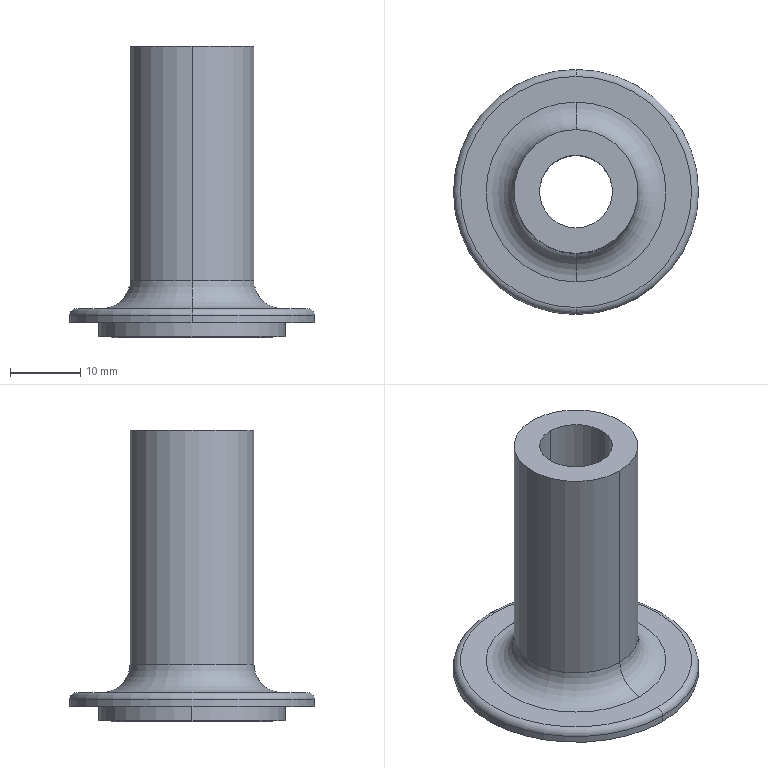Part | SolidWorks | features BaseBody 1 | 1 solid | 51 faces | box 35 x 35 x 41.7 mm | volume 8862 mm3 | torus 22 | cone 14 | cylinder 8 | plane 7 | commonest cylinder face diameters 10.4 x2 17.7 x2 26.6 x2 35 x2
STEP:
#1=CARTESIAN_POINT('',(1903.,34.85,823.));
#2=VERTEX_POINT('',#1);
#3=CARTESIAN_POINT('',(1903.,9.15,823.));
#4=VERTEX_POINT('',#3);
#5=CARTESIAN_POINT('',(1903.,22.,823.));
#6=DIRECTION('',(0.,0.,1.));
#7=DIRECTION('',(0.,1.,0.));
#8=AXIS2_PLACEMENT_3D('',#5,#6,#7);
#9=CIRCLE('',#8,12.85);
#10=EDGE_CURVE('',#2,#4,#9,.T.);
#11=ORIENTED_EDGE('',*,*,#10,.T.);
#12=CARTESIAN_POINT('',(1903.,13.15,827.));
#13=VERTEX_POINT('',#12);
#14=CARTESIAN_POINT('',(1903.,9.15,827.));
#15=DIRECTION('',(1.,0.,0.));
#16=DIRECTION('',(0.,1.,0.));
#17=AXIS2_PLACEMENT_3D('',#14,#15,#16);
#18=CIRCLE('',#17,4.);
#19=EDGE_CURVE('',#4,#13,#18,.T.);
#20=ORIENTED_EDGE('',*,*,#19,.T.);
#21=CARTESIAN_POINT('',(1903.,30.85,827.));
#22=VERTEX_POINT('',#21);
#23=CARTESIAN_POINT('',(1903.,22.,827.));
#24=DIRECTION('',(0.,0.,1.));
#25=DIRECTION('',(0.,1.,0.));
#26=AXIS2_PLACEMENT_3D('',#23,#24,#25);
#27=CIRCLE('',#26,8.85);
#28=EDGE_CURVE('',#22,#13,#27,.T.);
#29=ORIENTED_EDGE('',*,*,#28,.F.);
#30=CARTESIAN_POINT('',(1903.,34.85,827.));
#31=DIRECTION('',(1.,0.,0.));
#32=DIRECTION('',(0.,-1.,0.));
#33=AXIS2_PLACEMENT_3D('',#30,#31,#32);
#34=CIRCLE('',#33,4.);
#35=EDGE_CURVE('',#22,#2,#34,.T.);
#36=ORIENTED_EDGE('',*,*,#35,.T.);
#37=EDGE_LOOP('',(#11,#20,#29,#36));
#38=FACE_OUTER_BOUND('',#37,.T.);
#39=CARTESIAN_POINT('',(1903.,22.,827.));
#40=DIRECTION('',(0.,0.,1.));
#41=DIRECTION('',(0.,1.,0.));
#42=AXIS2_PLACEMENT_3D('',#39,#40,#41);
#43=TOROIDAL_SURFACE('',#42,12.85,4.);
#44=ADVANCED_FACE('',(#38),#43,.F.);
#45=CARTESIAN_POINT('',(1903.,22.,827.));
#46=DIRECTION('',(0.,0.,-1.));
#47=DIRECTION('',(0.,1.,0.));
#48=AXIS2_PLACEMENT_3D('',#45,#46,#47);
#49=CIRCLE('',#48,8.85);
#50=EDGE_CURVE('',#22,#13,#49,.T.);
#51=ORIENTED_EDGE('',*,*,#50,.T.);
#52=ORIENTED_EDGE('',*,*,#19,.F.);
#53=CARTESIAN_POINT('',(1903.,22.,823.));
#54=DIRECTION('',(0.,0.,-1.));
#55=DIRECTION('',(0.,1.,0.));
#56=AXIS2_PLACEMENT_3D('',#53,#54,#55);
#57=CIRCLE('',#56,12.85);
#58=EDGE_CURVE('',#2,#4,#57,.T.);
#59=ORIENTED_EDGE('',*,*,#58,.F.);
#60=ORIENTED_EDGE('',*,*,#35,.F.);
#61=EDGE_LOOP('',(#51,#52,#59,#60));
#62=FACE_OUTER_BOUND('',#61,.T.);
#63=CARTESIAN_POINT('',(1903.,22.,827.));
#64=DIRECTION('',(0.,0.,1.));
#65=DIRECTION('',(0.,1.,0.));
#66=AXIS2_PLACEMENT_3D('',#63,#64,#65);
#67=TOROIDAL_SURFACE('',#66,12.85,4.);
#68=ADVANCED_FACE('',(#62),#67,.F.);
#69=CARTESIAN_POINT('',(1903.,38.5,823.));
#70=VERTEX_POINT('',#69);
#71=CARTESIAN_POINT('',(1903.,5.5,823.));
#72=VERTEX_POINT('',#71);
#73=CARTESIAN_POINT('',(1903.,22.,823.));
#74=DIRECTION('',(0.,0.,-1.));
#75=DIRECTION('',(0.,1.,0.));
#76=AXIS2_PLACEMENT_3D('',#73,#74,#75);
#77=CIRCLE('',#76,16.5);
#78=EDGE_CURVE('',#70,#72,#77,.T.);
#79=ORIENTED_EDGE('',*,*,#78,.F.);
#80=CARTESIAN_POINT('',(1903.,22.,823.));
#81=DIRECTION('',(0.,0.,1.));
#82=DIRECTION('',(0.,1.,0.));
#83=AXIS2_PLACEMENT_3D('',#80,#81,#82);
#84=CIRCLE('',#83,16.5);
#85=EDGE_CURVE('',#70,#72,#84,.T.);
#86=ORIENTED_EDGE('',*,*,#85,.T.);
#87=EDGE_LOOP('',(#79,#86));
#88=FACE_OUTER_BOUND('',#87,.T.);
#89=ORIENTED_EDGE('',*,*,#10,.F.);
#90=ORIENTED_EDGE('',*,*,#58,.T.);
#91=EDGE_LOOP('',(#89,#90));
#92=FACE_BOUND('',#91,.T.);
#93=CARTESIAN_POINT('',(1903.,22.,823.));
#94=DIRECTION('',(0.,0.,1.));
#95=DIRECTION('',(0.,1.,0.));
#96=AXIS2_PLACEMENT_3D('',#93,#94,#95);
#97=PLANE('',#96);
#98=ADVANCED_FACE('',(#88,#92),#97,.T.);
#99=CARTESIAN_POINT('',(1903.,39.5,822.));
#100=VERTEX_POINT('',#99);
#101=CARTESIAN_POINT('',(1903.,4.5,822.));
#102=VERTEX_POINT('',#101);
#103=CARTESIAN_POINT('',(1903.,22.,822.));
#104=DIRECTION('',(0.,0.,1.));
#105=DIRECTION('',(0.,1.,0.));
#106=AXIS2_PLACEMENT_3D('',#103,#104,#105);
#107=CIRCLE('',#106,17.5);
#108=EDGE_CURVE('',#100,#102,#107,.T.);
#109=ORIENTED_EDGE('',*,*,#108,.T.);
#110=CARTESIAN_POINT('',(1903.,5.5,822.));
#111=DIRECTION('',(-1.,0.,0.));
#112=DIRECTION('',(0.,0.,1.));
#113=AXIS2_PLACEMENT_3D('',#110,#111,#112);
#114=CIRCLE('',#113,1.);
#115=EDGE_CURVE('',#102,#72,#114,.T.);
#116=ORIENTED_EDGE('',*,*,#115,.T.);
#117=ORIENTED_EDGE('',*,*,#85,.F.);
#118=CARTESIAN_POINT('',(1903.,38.5,822.));
#119=DIRECTION('',(-1.,0.,0.));
#120=DIRECTION('',(0.,0.,1.));
#121=AXIS2_PLACEMENT_3D('',#118,#119,#120);
#122=CIRCLE('',#121,1.);
#123=EDGE_CURVE('',#70,#100,#122,.T.);
#124=ORIENTED_EDGE('',*,*,#123,.T.);
#125=EDGE_LOOP('',(#109,#116,#117,#124));
#126=FACE_OUTER_BOUND('',#125,.T.);
#127=CARTESIAN_POINT('',(1903.,22.,822.));
#128=DIRECTION('',(0.,0.,1.));
#129=DIRECTION('',(0.,1.,0.));
#130=AXIS2_PLACEMENT_3D('',#127,#128,#129);
#131=TOROIDAL_SURFACE('',#130,16.5,1.);
#132=ADVANCED_FACE('',(#126),#131,.T.);
#133=ORIENTED_EDGE('',*,*,#78,.T.);
#134=ORIENTED_EDGE('',*,*,#115,.F.);
#135=CARTESIAN_POINT('',(1903.,22.,822.));
#136=DIRECTION('',(0.,0.,-1.));
#137=DIRECTION('',(0.,1.,0.));
#138=AXIS2_PLACEMENT_3D('',#135,#136,#137);
#139=CIRCLE('',#138,17.5);
#140=EDGE_CURVE('',#100,#102,#139,.T.);
#141=ORIENTED_EDGE('',*,*,#140,.F.);
#142=ORIENTED_EDGE('',*,*,#123,.F.);
#143=EDGE_LOOP('',(#133,#134,#141,#142));
#144=FACE_OUTER_BOUND('',#143,.T.);
#145=CARTESIAN_POINT('',(1903.,22.,822.));
#146=DIRECTION('',(0.,0.,1.));
#147=DIRECTION('',(0.,1.,0.));
#148=AXIS2_PLACEMENT_3D('',#145,#146,#147);
#149=TOROIDAL_SURFACE('',#148,16.5,1.);
#150=ADVANCED_FACE('',(#144),#149,.T.);
#151=CARTESIAN_POINT('',(1903.,39.5,821.));
#152=VERTEX_POINT('',#151);
#153=CARTESIAN_POINT('',(1903.,39.5,822.));
#154=DIRECTION('',(0.,0.,1.));
#155=VECTOR('',#154,1000.);
#156=LINE('',#153,#155);
#157=EDGE_CURVE('',#152,#100,#156,.T.);
#158=ORIENTED_EDGE('',*,*,#157,.T.);
#159=ORIENTED_EDGE('',*,*,#140,.T.);
#160=CARTESIAN_POINT('',(1903.,4.5,821.));
#161=VERTEX_POINT('',#160);
#162=CARTESIAN_POINT('',(1903.,4.5,822.));
#163=DIRECTION('',(0.,0.,-1.));
#164=VECTOR('',#163,1000.);
#165=LINE('',#162,#164);
#166=EDGE_CURVE('',#102,#161,#165,.T.);
#167=ORIENTED_EDGE('',*,*,#166,.T.);
#168=CARTESIAN_POINT('',(1903.,22.,821.));
#169=DIRECTION('',(0.,0.,-1.));
#170=DIRECTION('',(0.,1.,0.));
#171=AXIS2_PLACEMENT_3D('',#168,#169,#170);
#172=CIRCLE('',#171,17.5);
#173=EDGE_CURVE('',#152,#161,#172,.T.);
#174=ORIENTED_EDGE('',*,*,#173,.F.);
#175=EDGE_LOOP('',(#158,#159,#167,#174));
#176=FACE_OUTER_BOUND('',#175,.T.);
#177=CARTESIAN_POINT('',(1903.,22.,816.925));
#178=DIRECTION('',(0.,0.,1.));
#179=DIRECTION('',(0.,1.,0.));
#180=AXIS2_PLACEMENT_3D('',#177,#178,#179);
#181=CYLINDRICAL_SURFACE('',#180,17.5);
#182=ADVANCED_FACE('',(#176),#181,.T.);
#183=ORIENTED_EDGE('',*,*,#173,.T.);
#184=CARTESIAN_POINT('',(1903.,22.,821.));
#185=DIRECTION('',(0.,0.,-1.));
#186=DIRECTION('',(0.,-1.,0.));
#187=AXIS2_PLACEMENT_3D('',#184,#185,#186);
#188=CIRCLE('',#187,17.5);
#189=EDGE_CURVE('',#161,#152,#188,.T.);
#190=ORIENTED_EDGE('',*,*,#189,.T.);
#191=EDGE_LOOP('',(#183,#190));
#192=FACE_OUTER_BOUND('',#191,.T.);
#193=CARTESIAN_POINT('',(1916.3,22.,821.));
#194=VERTEX_POINT('',#193);
#195=CARTESIAN_POINT('',(1889.7,22.,821.));
#196=VERTEX_POINT('',#195);
#197=CARTESIAN_POINT('',(1903.,22.,821.));
#198=DIRECTION('',(0.,0.,1.));
#199=DIRECTION('',(1.,0.,0.));
#200=AXIS2_PLACEMENT_3D('',#197,#198,#199);
#201=CIRCLE('',#200,13.3);
#202=EDGE_CURVE('',#194,#196,#201,.T.);
#203=ORIENTED_EDGE('',*,*,#202,.T.);
#204=CARTESIAN_POINT('',(1903.,22.,821.));
#205=DIRECTION('',(0.,0.,-1.));
#206=DIRECTION('',(1.,0.,0.));
#207=AXIS2_PLACEMENT_3D('',#204,#205,#206);
#208=CIRCLE('',#207,13.3);
#209=EDGE_CURVE('',#194,#196,#208,.T.);
#210=ORIENTED_EDGE('',*,*,#209,.F.);
#211=EDGE_LOOP('',(#203,#210));
#212=FACE_BOUND('',#211,.T.);
#213=CARTESIAN_POINT('',(1903.,22.,821.));
#214=DIRECTION('',(0.,0.,-1.));
#215=DIRECTION('',(-1.,0.,0.));
#216=AXIS2_PLACEMENT_3D('',#213,#214,#215);
#217=PLANE('',#216);
#218=ADVANCED_FACE('',(#192,#212),#217,.T.);
#219=CARTESIAN_POINT('',(1916.3,22.,819.));
#220=VERTEX_POINT('',#219);
#221=CARTESIAN_POINT('',(1916.3,22.,819.));
#222=DIRECTION('',(0.,0.,-1.));
#223=VECTOR('',#222,1000.);
#224=LINE('',#221,#223);
#225=EDGE_CURVE('',#194,#220,#224,.T.);
#226=ORIENTED_EDGE('',*,*,#225,.F.);
#227=ORIENTED_EDGE('',*,*,#209,.T.);
#228=CARTESIAN_POINT('',(1889.7,22.,819.));
#229=VERTEX_POINT('',#228);
#230=CARTESIAN_POINT('',(1889.7,22.,819.));
#231=DIRECTION('',(0.,0.,1.));
#232=VECTOR('',#231,1000.);
#233=LINE('',#230,#232);
#234=EDGE_CURVE('',#229,#196,#233,.T.);
#235=ORIENTED_EDGE('',*,*,#234,.F.);
#236=CARTESIAN_POINT('',(1903.,22.,819.));
#237=DIRECTION('',(0.,0.,-1.));
#238=DIRECTION('',(1.,0.,0.));
#239=AXIS2_PLACEMENT_3D('',#236,#237,#238);
#240=CIRCLE('',#239,13.3);
#241=EDGE_CURVE('',#220,#229,#240,.T.);
#242=ORIENTED_EDGE('',*,*,#241,.F.);
#243=EDGE_LOOP('',(#226,#227,#235,#242));
#244=FACE_OUTER_BOUND('',#243,.T.);
#245=CARTESIAN_POINT('',(1903.,22.,821.1));
#246=DIRECTION('',(0.,0.,-1.));
#247=DIRECTION('',(-1.,0.,0.));
#248=AXIS2_PLACEMENT_3D('',#245,#246,#247);
#249=CYLINDRICAL_SURFACE('',#248,13.3);
#250=ADVANCED_FACE('',(#244),#249,.T.);
#251=CARTESIAN_POINT('',(1903.,22.,819.));
#252=DIRECTION('',(0.,0.,-1.));
#253=DIRECTION('',(-1.,0.,0.));
#254=AXIS2_PLACEMENT_3D('',#251,#252,#253);
#255=CIRCLE('',#254,13.3);
#256=EDGE_CURVE('',#229,#220,#255,.T.);
#257=ORIENTED_EDGE('',*,*,#256,.T.);
#258=ORIENTED_EDGE('',*,*,#241,.T.);
#259=EDGE_LOOP('',(#257,#258));
#260=FACE_OUTER_BOUND('',#259,.T.);
#261=CARTESIAN_POINT('',(1891.327,22.,819.));
#262=VERTEX_POINT('',#261);
#263=CARTESIAN_POINT('',(1914.673,22.,819.));
#264=VERTEX_POINT('',#263);
#265=CARTESIAN_POINT('',(1903.,22.,819.));
#266=DIRECTION('',(0.,0.,1.));
#267=DIRECTION('',(-1.,0.,0.));
#268=AXIS2_PLACEMENT_3D('',#265,#266,#267);
#269=CIRCLE('',#268,11.673);
#270=EDGE_CURVE('',#262,#264,#269,.T.);
#271=ORIENTED_EDGE('',*,*,#270,.T.);
#272=CARTESIAN_POINT('',(1903.,22.,819.));
#273=DIRECTION('',(0.,0.,1.));
#274=DIRECTION('',(1.,0.,0.));
#275=AXIS2_PLACEMENT_3D('',#272,#273,#274);
#276=CIRCLE('',#275,11.673);
#277=EDGE_CURVE('',#264,#262,#276,.T.);
#278=ORIENTED_EDGE('',*,*,#277,.T.);
#279=EDGE_LOOP('',(#271,#278));
#280=FACE_BOUND('',#279,.T.);
#281=CARTESIAN_POINT('',(1903.,22.,819.));
#282=DIRECTION('',(0.,0.,1.));
#283=DIRECTION('',(0.,1.,0.));
#284=AXIS2_PLACEMENT_3D('',#281,#282,#283);
#285=PLANE('',#284);
#286=ADVANCED_FACE('',(#260,#280),#285,.F.);
#287=CARTESIAN_POINT('',(1891.673,22.,819.));
#288=VERTEX_POINT('',#287);
#289=CARTESIAN_POINT('',(1914.327,22.,819.));
#290=VERTEX_POINT('',#289);
#291=CARTESIAN_POINT('',(1903.,22.,819.));
#292=DIRECTION('',(0.,0.,1.));
#293=DIRECTION('',(-1.,0.,0.));
#294=AXIS2_PLACEMENT_3D('',#291,#292,#293);
#295=CIRCLE('',#294,11.327);
#296=EDGE_CURVE('',#288,#290,#295,.T.);
#297=ORIENTED_EDGE('',*,*,#296,.F.);
#298=CARTESIAN_POINT('',(1903.,22.,819.));
#299=DIRECTION('',(0.,0.,1.));
#300=DIRECTION('',(1.,0.,0.));
#301=AXIS2_PLACEMENT_3D('',#298,#299,#300);
#302=CIRCLE('',#301,11.327);
#303=EDGE_CURVE('',#290,#288,#302,.T.);
#304=ORIENTED_EDGE('',*,*,#303,.F.);
#305=EDGE_LOOP('',(#297,#304));
#306=FACE_OUTER_BOUND('',#305,.T.);
#307=CARTESIAN_POINT('',(1893.327,22.,819.));
#308=VERTEX_POINT('',#307);
#309=CARTESIAN_POINT('',(1912.673,22.,819.));
#310=VERTEX_POINT('',#309);
#311=CARTESIAN_POINT('',(1903.,22.,819.));
#312=DIRECTION('',(0.,0.,1.));
#313=DIRECTION('',(-1.,0.,0.));
#314=AXIS2_PLACEMENT_3D('',#311,#312,#313);
#315=CIRCLE('',#314,9.673);
#316=EDGE_CURVE('',#308,#310,#315,.T.);
#317=ORIENTED_EDGE('',*,*,#316,.T.);
#318=CARTESIAN_POINT('',(1903.,22.,819.));
#319=DIRECTION('',(0.,0.,1.));
#320=DIRECTION('',(1.,0.,0.));
#321=AXIS2_PLACEMENT_3D('',#318,#319,#320);
#322=CIRCLE('',#321,9.673);
#323=EDGE_CURVE('',#310,#308,#322,.T.);
#324=ORIENTED_EDGE('',*,*,#323,.T.);
#325=EDGE_LOOP('',(#317,#324));
#326=FACE_BOUND('',#325,.T.);
#327=CARTESIAN_POINT('',(1903.,22.,819.));
#328=DIRECTION('',(0.,0.,1.));
#329=DIRECTION('',(0.,1.,0.));
#330=AXIS2_PLACEMENT_3D('',#327,#328,#329);
#331=PLANE('',#330);
#332=ADVANCED_FACE('',(#306,#326),#331,.F.);
#333=CARTESIAN_POINT('',(1893.673,22.,819.));
#334=VERTEX_POINT('',#333);
#335=CARTESIAN_POINT('',(1912.327,22.,819.));
#336=VERTEX_POINT('',#335);
#337=CARTESIAN_POINT('',(1903.,22.,819.));
#338=DIRECTION('',(0.,0.,1.));
#339=DIRECTION('',(-1.,0.,0.));
#340=AXIS2_PLACEMENT_3D('',#337,#338,#339);
#341=CIRCLE('',#340,9.327);
#342=EDGE_CURVE('',#334,#336,#341,.T.);
#343=ORIENTED_EDGE('',*,*,#342,.F.);
#344=CARTESIAN_POINT('',(1903.,22.,819.));
#345=DIRECTION('',(0.,0.,1.));
#346=DIRECTION('',(1.,0.,0.));
#347=AXIS2_PLACEMENT_3D('',#344,#345,#346);
#348=CIRCLE('',#347,9.327);
#349=EDGE_CURVE('',#336,#334,#348,.T.);
#350=ORIENTED_EDGE('',*,*,#349,.F.);
#351=EDGE_LOOP('',(#343,#350));
#352=FACE_OUTER_BOUND('',#351,.T.);
#353=CARTESIAN_POINT('',(1895.327,22.,819.));
#354=VERTEX_POINT('',#353);
#355=CARTESIAN_POINT('',(1910.673,22.,819.));
#356=VERTEX_POINT('',#355);
#357=CARTESIAN_POINT('',(1903.,22.,819.));
#358=DIRECTION('',(0.,0.,1.));
#359=DIRECTION('',(-1.,0.,0.));
#360=AXIS2_PLACEMENT_3D('',#357,#358,#359);
#361=CIRCLE('',#360,7.673);
#362=EDGE_CURVE('',#354,#356,#361,.T.);
#363=ORIENTED_EDGE('',*,*,#362,.T.);
#364=CARTESIAN_POINT('',(1903.,22.,819.));
#365=DIRECTION('',(0.,0.,1.));
#366=DIRECTION('',(1.,0.,0.));
#367=AXIS2_PLACEMENT_3D('',#364,#365,#366);
#368=CIRCLE('',#367,7.673);
#369=EDGE_CURVE('',#356,#354,#368,.T.);
#370=ORIENTED_EDGE('',*,*,#369,.T.);
#371=EDGE_LOOP('',(#363,#370));
#372=FACE_BOUND('',#371,.T.);
#373=CARTESIAN_POINT('',(1903.,22.,819.));
#374=DIRECTION('',(0.,0.,1.));
#375=DIRECTION('',(0.,1.,0.));
#376=AXIS2_PLACEMENT_3D('',#373,#374,#375);
#377=PLANE('',#376);
#378=ADVANCED_FACE('',(#352,#372),#377,.F.);
#379=CARTESIAN_POINT('',(1895.673,22.,819.));
#380=VERTEX_POINT('',#379);
#381=CARTESIAN_POINT('',(1910.327,22.,819.));
#382=VERTEX_POINT('',#381);
#383=CARTESIAN_POINT('',(1903.,22.,819.));
#384=DIRECTION('',(0.,0.,1.));
#385=DIRECTION('',(-1.,0.,0.));
#386=AXIS2_PLACEMENT_3D('',#383,#384,#385);
#387=CIRCLE('',#386,7.327);
#388=EDGE_CURVE('',#380,#382,#387,.T.);
#389=ORIENTED_EDGE('',*,*,#388,.F.);
#390=CARTESIAN_POINT('',(1903.,22.,819.));
#391=DIRECTION('',(0.,0.,1.));
#392=DIRECTION('',(1.,0.,0.));
#393=AXIS2_PLACEMENT_3D('',#390,#391,#392);
#394=CIRCLE('',#393,7.327);
#395=EDGE_CURVE('',#382,#380,#394,.T.);
#396=ORIENTED_EDGE('',*,*,#395,.F.);
#397=EDGE_LOOP('',(#389,#396));
#398=FACE_OUTER_BOUND('',#397,.T.);
#399=CARTESIAN_POINT('',(1903.,28.,819.));
#400=VERTEX_POINT('',#399);
#401=CARTESIAN_POINT('',(1903.,16.,819.));
#402=VERTEX_POINT('',#401);
#403=CARTESIAN_POINT('',(1903.,22.,819.));
#404=DIRECTION('',(0.,0.,-1.));
#405=DIRECTION('',(0.,1.,0.));
#406=AXIS2_PLACEMENT_3D('',#403,#404,#405);
#407=CIRCLE('',#406,6.);
#408=EDGE_CURVE('',#400,#402,#407,.T.);
#409=ORIENTED_EDGE('',*,*,#408,.F.);
#410=CARTESIAN_POINT('',(1903.,22.,819.));
#411=DIRECTION('',(0.,0.,1.));
#412=DIRECTION('',(0.,1.,0.));
#413=AXIS2_PLACEMENT_3D('',#410,#411,#412);
#414=CIRCLE('',#413,6.);
#415=EDGE_CURVE('',#400,#402,#414,.T.);
#416=ORIENTED_EDGE('',*,*,#415,.T.);
#417=EDGE_LOOP('',(#409,#416));
#418=FACE_BOUND('',#417,.T.);
#419=CARTESIAN_POINT('',(1903.,22.,819.));
#420=DIRECTION('',(0.,0.,1.));
#421=DIRECTION('',(0.,1.,0.));
#422=AXIS2_PLACEMENT_3D('',#419,#420,#421);
#423=PLANE('',#422);
#424=ADVANCED_FACE('',(#398,#418),#423,.F.);
#425=CARTESIAN_POINT('',(1903.,27.2,824.));
#426=VERTEX_POINT('',#425);
#427=CARTESIAN_POINT('',(1903.,16.8,824.));
#428=VERTEX_POINT('',#427);
#429=CARTESIAN_POINT('',(1903.,22.,824.));
#430=DIRECTION('',(0.,0.,1.));
#431=DIRECTION('',(0.,1.,0.));
#432=AXIS2_PLACEMENT_3D('',#429,#430,#431);
#433=CIRCLE('',#432,5.2);
#434=EDGE_CURVE('',#426,#428,#433,.T.);
#435=ORIENTED_EDGE('',*,*,#434,.T.);
#436=CARTESIAN_POINT('',(1903.,16.,819.));
#437=DIRECTION('',(0.,-0.158,-0.9874));
#438=VECTOR('',#437,1000.);
#439=LINE('',#436,#438);
#440=EDGE_CURVE('',#428,#402,#439,.T.);
#441=ORIENTED_EDGE('',*,*,#440,.T.);
#442=ORIENTED_EDGE('',*,*,#415,.F.);
#443=CARTESIAN_POINT('',(1903.,28.,819.));
#444=DIRECTION('',(0.,-0.158,0.9874));
#445=VECTOR('',#444,1000.);
#446=LINE('',#443,#445);
#447=EDGE_CURVE('',#400,#426,#446,.T.);
#448=ORIENTED_EDGE('',*,*,#447,.T.);
#449=EDGE_LOOP('',(#435,#441,#442,#448));
#450=FACE_OUTER_BOUND('',#449,.T.);
#451=CARTESIAN_POINT('',(1903.,22.,821.5));
#452=DIRECTION('',(0.,0.,-1.));
#453=DIRECTION('',(0.,-1.,0.));
#454=AXIS2_PLACEMENT_3D('',#451,#452,#453);
#455=CONICAL_SURFACE('',#454,5.6,0.1587);
#456=ADVANCED_FACE('',(#450),#455,.F.);
#457=ORIENTED_EDGE('',*,*,#408,.T.);
#458=ORIENTED_EDGE('',*,*,#440,.F.);
#459=CARTESIAN_POINT('',(1903.,22.,824.));
#460=DIRECTION('',(0.,0.,-1.));
#461=DIRECTION('',(0.,1.,0.));
#462=AXIS2_PLACEMENT_3D('',#459,#460,#461);
#463=CIRCLE('',#462,5.2);
#464=EDGE_CURVE('',#426,#428,#463,.T.);
#465=ORIENTED_EDGE('',*,*,#464,.F.);
#466=ORIENTED_EDGE('',*,*,#447,.F.);
#467=EDGE_LOOP('',(#457,#458,#465,#466));
#468=FACE_OUTER_BOUND('',#467,.T.);
#469=CARTESIAN_POINT('',(1903.,22.,821.5));
#470=DIRECTION('',(0.,0.,-1.));
#471=DIRECTION('',(0.,-1.,0.));
#472=AXIS2_PLACEMENT_3D('',#469,#470,#471);
#473=CONICAL_SURFACE('',#472,5.6,0.1587);
#474=ADVANCED_FACE('',(#468),#473,.F.);
#475=ORIENTED_EDGE('',*,*,#464,.T.);
#476=CARTESIAN_POINT('',(1903.,16.8,860.5));
#477=VERTEX_POINT('',#476);
#478=CARTESIAN_POINT('',(1903.,16.8,824.));
#479=DIRECTION('',(0.,0.,-1.));
#480=VECTOR('',#479,1000.);
#481=LINE('',#478,#480);
#482=EDGE_CURVE('',#477,#428,#481,.T.);
#483=ORIENTED_EDGE('',*,*,#482,.F.);
#484=CARTESIAN_POINT('',(1903.,27.2,860.5));
#485=VERTEX_POINT('',#484);
#486=CARTESIAN_POINT('',(1903.,22.,860.5));
#487=DIRECTION('',(0.,0.,-1.));
#488=DIRECTION('',(0.,1.,0.));
#489=AXIS2_PLACEMENT_3D('',#486,#487,#488);
#490=CIRCLE('',#489,5.2);
#491=EDGE_CURVE('',#485,#477,#490,.T.);
#492=ORIENTED_EDGE('',*,*,#491,.F.);
#493=CARTESIAN_POINT('',(1903.,27.2,824.));
#494=DIRECTION('',(0.,0.,1.));
#495=VECTOR('',#494,1000.);
#496=LINE('',#493,#495);
#497=EDGE_CURVE('',#426,#485,#496,.T.);
#498=ORIENTED_EDGE('',*,*,#497,.F.);
#499=EDGE_LOOP('',(#475,#483,#492,#498));
#500=FACE_OUTER_BOUND('',#499,.T.);
#501=CARTESIAN_POINT('',(1903.,22.,816.925));
#502=DIRECTION('',(0.,0.,1.));
#503=DIRECTION('',(0.,1.,0.));
#504=AXIS2_PLACEMENT_3D('',#501,#502,#503);
#505=CYLINDRICAL_SURFACE('',#504,5.2);
#506=ADVANCED_FACE('',(#500),#505,.F.);
#507=CARTESIAN_POINT('',(1903.,22.,860.5));
#508=DIRECTION('',(0.,0.,1.));
#509=DIRECTION('',(0.,1.,0.));
#510=AXIS2_PLACEMENT_3D('',#507,#508,#509);
#511=CIRCLE('',#510,5.2);
#512=EDGE_CURVE('',#485,#477,#511,.T.);
#513=ORIENTED_EDGE('',*,*,#512,.T.);
#514=ORIENTED_EDGE('',*,*,#482,.T.);
#515=ORIENTED_EDGE('',*,*,#434,.F.);
#516=ORIENTED_EDGE('',*,*,#497,.T.);
#517=EDGE_LOOP('',(#513,#514,#515,#516));
#518=FACE_OUTER_BOUND('',#517,.T.);
#519=CARTESIAN_POINT('',(1903.,22.,816.925));
#520=DIRECTION('',(0.,0.,1.));
#521=DIRECTION('',(0.,1.,0.));
#522=AXIS2_PLACEMENT_3D('',#519,#520,#521);
#523=CYLINDRICAL_SURFACE('',#522,5.2);
#524=ADVANCED_FACE('',(#518),#523,.F.);
#525=CARTESIAN_POINT('',(1903.,30.85,860.5));
#526=VERTEX_POINT('',#525);
#527=CARTESIAN_POINT('',(1903.,13.15,860.5));
#528=VERTEX_POINT('',#527);
#529=CARTESIAN_POINT('',(1903.,22.,860.5));
#530=DIRECTION('',(0.,0.,-1.));
#531=DIRECTION('',(0.,1.,0.));
#532=AXIS2_PLACEMENT_3D('',#529,#530,#531);
#533=CIRCLE('',#532,8.85);
#534=EDGE_CURVE('',#526,#528,#533,.T.);
#535=ORIENTED_EDGE('',*,*,#534,.F.);
#536=CARTESIAN_POINT('',(1903.,22.,860.5));
#537=DIRECTION('',(0.,0.,1.));
#538=DIRECTION('',(0.,1.,0.));
#539=AXIS2_PLACEMENT_3D('',#536,#537,#538);
#540=CIRCLE('',#539,8.85);
#541=EDGE_CURVE('',#526,#528,#540,.T.);
#542=ORIENTED_EDGE('',*,*,#541,.T.);
#543=EDGE_LOOP('',(#535,#542));
#544=FACE_OUTER_BOUND('',#543,.T.);
#545=ORIENTED_EDGE('',*,*,#512,.F.);
#546=ORIENTED_EDGE('',*,*,#491,.T.);
#547=EDGE_LOOP('',(#545,#546));
#548=FACE_BOUND('',#547,.T.);
#549=CARTESIAN_POINT('',(1903.,22.,860.5));
#550=DIRECTION('',(0.,0.,1.));
#551=DIRECTION('',(0.,1.,0.));
#552=AXIS2_PLACEMENT_3D('',#549,#550,#551);
#553=PLANE('',#552);
#554=ADVANCED_FACE('',(#544,#548),#553,.T.);
#555=ORIENTED_EDGE('',*,*,#28,.T.);
#556=CARTESIAN_POINT('',(1903.,13.15,860.5));
#557=DIRECTION('',(0.,0.,-1.));
#558=VECTOR('',#557,1000.);
#559=LINE('',#556,#558);
#560=EDGE_CURVE('',#528,#13,#559,.T.);
#561=ORIENTED_EDGE('',*,*,#560,.F.);
#562=ORIENTED_EDGE('',*,*,#541,.F.);
#563=CARTESIAN_POINT('',(1903.,30.85,860.5));
#564=DIRECTION('',(0.,0.,1.));
#565=VECTOR('',#564,1000.);
#566=LINE('',#563,#565);
#567=EDGE_CURVE('',#22,#526,#566,.T.);
#568=ORIENTED_EDGE('',*,*,#567,.F.);
#569=EDGE_LOOP('',(#555,#561,#562,#568));
#570=FACE_OUTER_BOUND('',#569,.T.);
#571=CARTESIAN_POINT('',(1903.,22.,816.925));
#572=DIRECTION('',(0.,0.,1.));
#573=DIRECTION('',(0.,1.,0.));
#574=AXIS2_PLACEMENT_3D('',#571,#572,#573);
#575=CYLINDRICAL_SURFACE('',#574,8.85);
#576=ADVANCED_FACE('',(#570),#575,.T.);
#577=ORIENTED_EDGE('',*,*,#534,.T.);
#578=ORIENTED_EDGE('',*,*,#560,.T.);
#579=ORIENTED_EDGE('',*,*,#50,.F.);
#580=ORIENTED_EDGE('',*,*,#567,.T.);
#581=EDGE_LOOP('',(#577,#578,#579,#580));
#582=FACE_OUTER_BOUND('',#581,.T.);
#583=CARTESIAN_POINT('',(1903.,22.,816.925));
#584=DIRECTION('',(0.,0.,1.));
#585=DIRECTION('',(0.,1.,0.));
#586=AXIS2_PLACEMENT_3D('',#583,#584,#585);
#587=CYLINDRICAL_SURFACE('',#586,8.85);
#588=ADVANCED_FACE('',(#582),#587,.T.);
#589=ORIENTED_EDGE('',*,*,#234,.T.);
#590=ORIENTED_EDGE('',*,*,#202,.F.);
#591=ORIENTED_EDGE('',*,*,#225,.T.);
#592=ORIENTED_EDGE('',*,*,#256,.F.);
#593=EDGE_LOOP('',(#589,#590,#591,#592));
#594=FACE_OUTER_BOUND('',#593,.T.);
#595=CARTESIAN_POINT('',(1903.,22.,821.1));
#596=DIRECTION('',(0.,0.,-1.));
#597=DIRECTION('',(-1.,0.,0.));
#598=AXIS2_PLACEMENT_3D('',#595,#596,#597);
#599=CYLINDRICAL_SURFACE('',#598,13.3);
#600=ADVANCED_FACE('',(#594),#599,.T.);
#601=CARTESIAN_POINT('',(1891.63,22.,818.975));
#602=VERTEX_POINT('',#601);
#603=CARTESIAN_POINT('',(1891.673,22.,818.95));
#604=DIRECTION('',(0.,-1.,0.));
#605=DIRECTION('',(-0.866,0.,0.5));
#606=AXIS2_PLACEMENT_3D('',#603,#604,#605);
#607=CIRCLE('',#606,0.05);
#608=EDGE_CURVE('',#288,#602,#607,.T.);
#609=ORIENTED_EDGE('',*,*,#608,.T.);
#610=CARTESIAN_POINT('',(1914.37,22.,818.975));
#611=VERTEX_POINT('',#610);
#612=CARTESIAN_POINT('',(1903.,22.,818.975));
#613=DIRECTION('',(0.,0.,1.));
#614=DIRECTION('',(1.,0.,0.));
#615=AXIS2_PLACEMENT_3D('',#612,#613,#614);
#616=CIRCLE('',#615,11.37);
#617=EDGE_CURVE('',#611,#602,#616,.T.);
#618=ORIENTED_EDGE('',*,*,#617,.F.);
#619=CARTESIAN_POINT('',(1914.327,22.,818.95));
#620=DIRECTION('',(0.,-1.,0.));
#621=DIRECTION('',(0.866,0.,0.5));
#622=AXIS2_PLACEMENT_3D('',#619,#620,#621);
#623=CIRCLE('',#622,0.05);
#624=EDGE_CURVE('',#611,#290,#623,.T.);
#625=ORIENTED_EDGE('',*,*,#624,.T.);
#626=ORIENTED_EDGE('',*,*,#303,.T.);
#627=EDGE_LOOP('',(#609,#618,#625,#626));
#628=FACE_OUTER_BOUND('',#627,.T.);
#629=CARTESIAN_POINT('',(1903.,22.,818.95));
#630=DIRECTION('',(0.,0.,1.));
#631=DIRECTION('',(1.,0.,0.));
#632=AXIS2_PLACEMENT_3D('',#629,#630,#631);
#633=TOROIDAL_SURFACE('',#632,11.327,0.05);
#634=ADVANCED_FACE('',(#628),#633,.F.);
#635=ORIENTED_EDGE('',*,*,#624,.F.);
#636=CARTESIAN_POINT('',(1903.,22.,818.975));
#637=DIRECTION('',(0.,0.,-1.));
#638=DIRECTION('',(1.,0.,0.));
#639=AXIS2_PLACEMENT_3D('',#636,#637,#638);
#640=CIRCLE('',#639,11.37);
#641=EDGE_CURVE('',#611,#602,#640,.T.);
#642=ORIENTED_EDGE('',*,*,#641,.T.);
#643=ORIENTED_EDGE('',*,*,#608,.F.);
#644=ORIENTED_EDGE('',*,*,#296,.T.);
#645=EDGE_LOOP('',(#635,#642,#643,#644));
#646=FACE_OUTER_BOUND('',#645,.T.);
#647=CARTESIAN_POINT('',(1903.,22.,818.95));
#648=DIRECTION('',(0.,0.,1.));
#649=DIRECTION('',(1.,0.,0.));
#650=AXIS2_PLACEMENT_3D('',#647,#648,#649);
#651=TOROIDAL_SURFACE('',#650,11.327,0.05);
#652=ADVANCED_FACE('',(#646),#651,.F.);
#653=CARTESIAN_POINT('',(1914.457,22.,818.825));
#654=VERTEX_POINT('',#653);
#655=CARTESIAN_POINT('',(1891.543,22.,818.825));
#656=VERTEX_POINT('',#655);
#657=CARTESIAN_POINT('',(1903.,22.,818.825));
#658=DIRECTION('',(0.,0.,-1.));
#659=DIRECTION('',(1.,0.,0.));
#660=AXIS2_PLACEMENT_3D('',#657,#658,#659);
#661=CIRCLE('',#660,11.457);
#662=EDGE_CURVE('',#654,#656,#661,.T.);
#663=ORIENTED_EDGE('',*,*,#662,.T.);
#664=CARTESIAN_POINT('',(1891.543,22.,818.825));
#665=DIRECTION('',(-0.5,0.,-0.866));
#666=VECTOR('',#665,1000.);
#667=LINE('',#664,#666);
#668=EDGE_CURVE('',#602,#656,#667,.T.);
#669=ORIENTED_EDGE('',*,*,#668,.F.);
#670=ORIENTED_EDGE('',*,*,#641,.F.);
#671=CARTESIAN_POINT('',(1914.457,22.,818.825));
#672=DIRECTION('',(-0.5,0.,0.866));
#673=VECTOR('',#672,1000.);
#674=LINE('',#671,#673);
#675=EDGE_CURVE('',#654,#611,#674,.T.);
#676=ORIENTED_EDGE('',*,*,#675,.F.);
#677=EDGE_LOOP('',(#663,#669,#670,#676));
#678=FACE_OUTER_BOUND('',#677,.T.);
#679=CARTESIAN_POINT('',(1903.,22.,818.9));
#680=DIRECTION('',(0.,0.,-1.));
#681=DIRECTION('',(-1.,0.,0.));
#682=AXIS2_PLACEMENT_3D('',#679,#680,#681);
#683=CONICAL_SURFACE('',#682,11.413,0.5236);
#684=ADVANCED_FACE('',(#678),#683,.F.);
#685=ORIENTED_EDGE('',*,*,#617,.T.);
#686=ORIENTED_EDGE('',*,*,#668,.T.);
#687=CARTESIAN_POINT('',(1903.,22.,818.825));
#688=DIRECTION('',(0.,0.,1.));
#689=DIRECTION('',(1.,0.,0.));
#690=AXIS2_PLACEMENT_3D('',#687,#688,#689);
#691=CIRCLE('',#690,11.457);
#692=EDGE_CURVE('',#654,#656,#691,.T.);
#693=ORIENTED_EDGE('',*,*,#692,.F.);
#694=ORIENTED_EDGE('',*,*,#675,.T.);
#695=EDGE_LOOP('',(#685,#686,#693,#694));
#696=FACE_OUTER_BOUND('',#695,.T.);
#697=CARTESIAN_POINT('',(1903.,22.,818.9));
#698=DIRECTION('',(0.,0.,-1.));
#699=DIRECTION('',(-1.,0.,0.));
#700=AXIS2_PLACEMENT_3D('',#697,#698,#699);
#701=CONICAL_SURFACE('',#700,11.413,0.5236);
#702=ADVANCED_FACE('',(#696),#701,.F.);
#703=ORIENTED_EDGE('',*,*,#692,.T.);
#704=CARTESIAN_POINT('',(1891.457,22.,818.825));
#705=VERTEX_POINT('',#704);
#706=CARTESIAN_POINT('',(1891.5,22.,818.85));
#707=DIRECTION('',(0.,1.,0.));
#708=DIRECTION('',(-0.866,0.,-0.5));
#709=AXIS2_PLACEMENT_3D('',#706,#707,#708);
#710=CIRCLE('',#709,0.05);
#711=EDGE_CURVE('',#656,#705,#710,.T.);
#712=ORIENTED_EDGE('',*,*,#711,.T.);
#713=CARTESIAN_POINT('',(1914.543,22.,818.825));
#714=VERTEX_POINT('',#713);
#715=CARTESIAN_POINT('',(1903.,22.,818.825));
#716=DIRECTION('',(0.,0.,1.));
#717=DIRECTION('',(1.,0.,0.));
#718=AXIS2_PLACEMENT_3D('',#715,#716,#717);
#719=CIRCLE('',#718,11.543);
#720=EDGE_CURVE('',#714,#705,#719,.T.);
#721=ORIENTED_EDGE('',*,*,#720,.F.);
#722=CARTESIAN_POINT('',(1914.5,22.,818.85));
#723=DIRECTION('',(0.,1.,0.));
#724=DIRECTION('',(0.866,0.,-0.5));
#725=AXIS2_PLACEMENT_3D('',#722,#723,#724);
#726=CIRCLE('',#725,0.05);
#727=EDGE_CURVE('',#714,#654,#726,.T.);
#728=ORIENTED_EDGE('',*,*,#727,.T.);
#729=EDGE_LOOP('',(#703,#712,#721,#728));
#730=FACE_OUTER_BOUND('',#729,.T.);
#731=CARTESIAN_POINT('',(1903.,22.,818.85));
#732=DIRECTION('',(0.,0.,1.));
#733=DIRECTION('',(1.,0.,0.));
#734=AXIS2_PLACEMENT_3D('',#731,#732,#733);
#735=TOROIDAL_SURFACE('',#734,11.5,0.05);
#736=ADVANCED_FACE('',(#730),#735,.T.);
#737=CARTESIAN_POINT('',(1903.,22.,818.825));
#738=DIRECTION('',(0.,0.,-1.));
#739=DIRECTION('',(1.,0.,0.));
#740=AXIS2_PLACEMENT_3D('',#737,#738,#739);
#741=CIRCLE('',#740,11.543);
#742=EDGE_CURVE('',#714,#705,#741,.T.);
#743=ORIENTED_EDGE('',*,*,#742,.T.);
#744=ORIENTED_EDGE('',*,*,#711,.F.);
#745=ORIENTED_EDGE('',*,*,#662,.F.);
#746=ORIENTED_EDGE('',*,*,#727,.F.);
#747=EDGE_LOOP('',(#743,#744,#745,#746));
#748=FACE_OUTER_BOUND('',#747,.T.);
#749=CARTESIAN_POINT('',(1903.,22.,818.85));
#750=DIRECTION('',(0.,0.,1.));
#751=DIRECTION('',(1.,0.,0.));
#752=AXIS2_PLACEMENT_3D('',#749,#750,#751);
#753=TOROIDAL_SURFACE('',#752,11.5,0.05);
#754=ADVANCED_FACE('',(#748),#753,.T.);
#755=CARTESIAN_POINT('',(1914.63,22.,818.975));
#756=VERTEX_POINT('',#755);
#757=CARTESIAN_POINT('',(1891.37,22.,818.975));
#758=VERTEX_POINT('',#757);
#759=CARTESIAN_POINT('',(1903.,22.,818.975));
#760=DIRECTION('',(0.,0.,-1.));
#761=DIRECTION('',(1.,0.,0.));
#762=AXIS2_PLACEMENT_3D('',#759,#760,#761);
#763=CIRCLE('',#762,11.63);
#764=EDGE_CURVE('',#756,#758,#763,.T.);
#765=ORIENTED_EDGE('',*,*,#764,.T.);
#766=CARTESIAN_POINT('',(1891.37,22.,818.975));
#767=DIRECTION('',(0.5,0.,-0.866));
#768=VECTOR('',#767,1000.);
#769=LINE('',#766,#768);
#770=EDGE_CURVE('',#758,#705,#769,.T.);
#771=ORIENTED_EDGE('',*,*,#770,.T.);
#772=ORIENTED_EDGE('',*,*,#742,.F.);
#773=CARTESIAN_POINT('',(1914.63,22.,818.975));
#774=DIRECTION('',(0.5,0.,0.866));
#775=VECTOR('',#774,1000.);
#776=LINE('',#773,#775);
#777=EDGE_CURVE('',#714,#756,#776,.T.);
#778=ORIENTED_EDGE('',*,*,#777,.T.);
#779=EDGE_LOOP('',(#765,#771,#772,#778));
#780=FACE_OUTER_BOUND('',#779,.T.);
#781=CARTESIAN_POINT('',(1903.,22.,818.9));
#782=DIRECTION('',(0.,0.,1.));
#783=DIRECTION('',(1.,0.,0.));
#784=AXIS2_PLACEMENT_3D('',#781,#782,#783);
#785=CONICAL_SURFACE('',#784,11.587,0.5236);
#786=ADVANCED_FACE('',(#780),#785,.T.);
#787=ORIENTED_EDGE('',*,*,#720,.T.);
#788=ORIENTED_EDGE('',*,*,#770,.F.);
#789=CARTESIAN_POINT('',(1903.,22.,818.975));
#790=DIRECTION('',(0.,0.,1.));
#791=DIRECTION('',(1.,0.,0.));
#792=AXIS2_PLACEMENT_3D('',#789,#790,#791);
#793=CIRCLE('',#792,11.63);
#794=EDGE_CURVE('',#756,#758,#793,.T.);
#795=ORIENTED_EDGE('',*,*,#794,.F.);
#796=ORIENTED_EDGE('',*,*,#777,.F.);
#797=EDGE_LOOP('',(#787,#788,#795,#796));
#798=FACE_OUTER_BOUND('',#797,.T.);
#799=CARTESIAN_POINT('',(1903.,22.,818.9));
#800=DIRECTION('',(0.,0.,1.));
#801=DIRECTION('',(1.,0.,0.));
#802=AXIS2_PLACEMENT_3D('',#799,#800,#801);
#803=CONICAL_SURFACE('',#802,11.587,0.5236);
#804=ADVANCED_FACE('',(#798),#803,.T.);
#805=CARTESIAN_POINT('',(1914.673,22.,818.95));
#806=DIRECTION('',(0.,1.,0.));
#807=DIRECTION('',(0.,0.,1.));
#808=AXIS2_PLACEMENT_3D('',#805,#806,#807);
#809=CIRCLE('',#808,0.05);
#810=EDGE_CURVE('',#756,#264,#809,.T.);
#811=ORIENTED_EDGE('',*,*,#810,.F.);
#812=ORIENTED_EDGE('',*,*,#794,.T.);
#813=CARTESIAN_POINT('',(1891.327,22.,818.95));
#814=DIRECTION('',(0.,1.,0.));
#815=DIRECTION('',(0.,0.,1.));
#816=AXIS2_PLACEMENT_3D('',#813,#814,#815);
#817=CIRCLE('',#816,0.05);
#818=EDGE_CURVE('',#262,#758,#817,.T.);
#819=ORIENTED_EDGE('',*,*,#818,.F.);
#820=ORIENTED_EDGE('',*,*,#277,.F.);
#821=EDGE_LOOP('',(#811,#812,#819,#820));
#822=FACE_OUTER_BOUND('',#821,.T.);
#823=CARTESIAN_POINT('',(1903.,22.,818.95));
#824=DIRECTION('',(0.,0.,1.));
#825=DIRECTION('',(1.,0.,0.));
#826=AXIS2_PLACEMENT_3D('',#823,#824,#825);
#827=TOROIDAL_SURFACE('',#826,11.673,0.05);
#828=ADVANCED_FACE('',(#822),#827,.F.);
#829=ORIENTED_EDGE('',*,*,#818,.T.);
#830=ORIENTED_EDGE('',*,*,#764,.F.);
#831=ORIENTED_EDGE('',*,*,#810,.T.);
#832=ORIENTED_EDGE('',*,*,#270,.F.);
#833=EDGE_LOOP('',(#829,#830,#831,#832));
#834=FACE_OUTER_BOUND('',#833,.T.);
#835=CARTESIAN_POINT('',(1903.,22.,818.95));
#836=DIRECTION('',(0.,0.,1.));
#837=DIRECTION('',(1.,0.,0.));
#838=AXIS2_PLACEMENT_3D('',#835,#836,#837);
#839=TOROIDAL_SURFACE('',#838,11.673,0.05);
#840=ADVANCED_FACE('',(#834),#839,.F.);
#841=CARTESIAN_POINT('',(1893.63,22.,818.975));
#842=VERTEX_POINT('',#841);
#843=CARTESIAN_POINT('',(1893.673,22.,818.95));
#844=DIRECTION('',(0.,-1.,0.));
#845=DIRECTION('',(-0.866,0.,0.5));
#846=AXIS2_PLACEMENT_3D('',#843,#844,#845);
#847=CIRCLE('',#846,0.05);
#848=EDGE_CURVE('',#334,#842,#847,.T.);
#849=ORIENTED_EDGE('',*,*,#848,.T.);
#850=CARTESIAN_POINT('',(1912.37,22.,818.975));
#851=VERTEX_POINT('',#850);
#852=CARTESIAN_POINT('',(1903.,22.,818.975));
#853=DIRECTION('',(0.,0.,1.));
#854=DIRECTION('',(1.,0.,0.));
#855=AXIS2_PLACEMENT_3D('',#852,#853,#854);
#856=CIRCLE('',#855,9.37);
#857=EDGE_CURVE('',#851,#842,#856,.T.);
#858=ORIENTED_EDGE('',*,*,#857,.F.);
#859=CARTESIAN_POINT('',(1912.327,22.,818.95));
#860=DIRECTION('',(0.,-1.,0.));
#861=DIRECTION('',(0.866,0.,0.5));
#862=AXIS2_PLACEMENT_3D('',#859,#860,#861);
#863=CIRCLE('',#862,0.05);
#864=EDGE_CURVE('',#851,#336,#863,.T.);
#865=ORIENTED_EDGE('',*,*,#864,.T.);
#866=ORIENTED_EDGE('',*,*,#349,.T.);
#867=EDGE_LOOP('',(#849,#858,#865,#866));
#868=FACE_OUTER_BOUND('',#867,.T.);
#869=CARTESIAN_POINT('',(1903.,22.,818.95));
#870=DIRECTION('',(0.,0.,1.));
#871=DIRECTION('',(1.,0.,0.));
#872=AXIS2_PLACEMENT_3D('',#869,#870,#871);
#873=TOROIDAL_SURFACE('',#872,9.327,0.05);
#874=ADVANCED_FACE('',(#868),#873,.F.);
#875=ORIENTED_EDGE('',*,*,#864,.F.);
#876=CARTESIAN_POINT('',(1903.,22.,818.975));
#877=DIRECTION('',(0.,0.,-1.));
#878=DIRECTION('',(1.,0.,0.));
#879=AXIS2_PLACEMENT_3D('',#876,#877,#878);
#880=CIRCLE('',#879,9.37);
#881=EDGE_CURVE('',#851,#842,#880,.T.);
#882=ORIENTED_EDGE('',*,*,#881,.T.);
#883=ORIENTED_EDGE('',*,*,#848,.F.);
#884=ORIENTED_EDGE('',*,*,#342,.T.);
#885=EDGE_LOOP('',(#875,#882,#883,#884));
#886=FACE_OUTER_BOUND('',#885,.T.);
#887=CARTESIAN_POINT('',(1903.,22.,818.95));
#888=DIRECTION('',(0.,0.,1.));
#889=DIRECTION('',(1.,0.,0.));
#890=AXIS2_PLACEMENT_3D('',#887,#888,#889);
#891=TOROIDAL_SURFACE('',#890,9.327,0.05);
#892=ADVANCED_FACE('',(#886),#891,.F.);
#893=CARTESIAN_POINT('',(1912.457,22.,818.825));
#894=VERTEX_POINT('',#893);
#895=CARTESIAN_POINT('',(1893.543,22.,818.825));
#896=VERTEX_POINT('',#895);
#897=CARTESIAN_POINT('',(1903.,22.,818.825));
#898=DIRECTION('',(0.,0.,-1.));
#899=DIRECTION('',(1.,0.,0.));
#900=AXIS2_PLACEMENT_3D('',#897,#898,#899);
#901=CIRCLE('',#900,9.457);
#902=EDGE_CURVE('',#894,#896,#901,.T.);
#903=ORIENTED_EDGE('',*,*,#902,.T.);
#904=CARTESIAN_POINT('',(1893.543,22.,818.825));
#905=DIRECTION('',(0.5,0.,0.866));
#906=VECTOR('',#905,1000.);
#907=LINE('',#904,#906);
#908=EDGE_CURVE('',#896,#842,#907,.T.);
#909=ORIENTED_EDGE('',*,*,#908,.T.);
#910=ORIENTED_EDGE('',*,*,#881,.F.);
#911=CARTESIAN_POINT('',(1912.457,22.,818.825));
#912=DIRECTION('',(0.5,0.,-0.866));
#913=VECTOR('',#912,1000.);
#914=LINE('',#911,#913);
#915=EDGE_CURVE('',#851,#894,#914,.T.);
#916=ORIENTED_EDGE('',*,*,#915,.T.);
#917=EDGE_LOOP('',(#903,#909,#910,#916));
#918=FACE_OUTER_BOUND('',#917,.T.);
#919=CARTESIAN_POINT('',(1903.,22.,818.9));
#920=DIRECTION('',(0.,0.,-1.));
#921=DIRECTION('',(-1.,0.,0.));
#922=AXIS2_PLACEMENT_3D('',#919,#920,#921);
#923=CONICAL_SURFACE('',#922,9.413,0.5236);
#924=ADVANCED_FACE('',(#918),#923,.F.);
#925=ORIENTED_EDGE('',*,*,#857,.T.);
#926=ORIENTED_EDGE('',*,*,#908,.F.);
#927=CARTESIAN_POINT('',(1903.,22.,818.825));
#928=DIRECTION('',(0.,0.,1.));
#929=DIRECTION('',(1.,0.,0.));
#930=AXIS2_PLACEMENT_3D('',#927,#928,#929);
#931=CIRCLE('',#930,9.457);
#932=EDGE_CURVE('',#894,#896,#931,.T.);
#933=ORIENTED_EDGE('',*,*,#932,.F.);
#934=ORIENTED_EDGE('',*,*,#915,.F.);
#935=EDGE_LOOP('',(#925,#926,#933,#934));
#936=FACE_OUTER_BOUND('',#935,.T.);
#937=CARTESIAN_POINT('',(1903.,22.,818.9));
#938=DIRECTION('',(0.,0.,-1.));
#939=DIRECTION('',(-1.,0.,0.));
#940=AXIS2_PLACEMENT_3D('',#937,#938,#939);
#941=CONICAL_SURFACE('',#940,9.413,0.5236);
#942=ADVANCED_FACE('',(#936),#941,.F.);
#943=ORIENTED_EDGE('',*,*,#932,.T.);
#944=CARTESIAN_POINT('',(1893.457,22.,818.825));
#945=VERTEX_POINT('',#944);
#946=CARTESIAN_POINT('',(1893.5,22.,818.85));
#947=DIRECTION('',(0.,-1.,0.));
#948=DIRECTION('',(-0.866,0.,-0.5));
#949=AXIS2_PLACEMENT_3D('',#946,#947,#948);
#950=CIRCLE('',#949,0.05);
#951=EDGE_CURVE('',#945,#896,#950,.T.);
#952=ORIENTED_EDGE('',*,*,#951,.F.);
#953=CARTESIAN_POINT('',(1912.543,22.,818.825));
#954=VERTEX_POINT('',#953);
#955=CARTESIAN_POINT('',(1903.,22.,818.825));
#956=DIRECTION('',(0.,0.,1.));
#957=DIRECTION('',(1.,0.,0.));
#958=AXIS2_PLACEMENT_3D('',#955,#956,#957);
#959=CIRCLE('',#958,9.543);
#960=EDGE_CURVE('',#954,#945,#959,.T.);
#961=ORIENTED_EDGE('',*,*,#960,.F.);
#962=CARTESIAN_POINT('',(1912.5,22.,818.85));
#963=DIRECTION('',(0.,-1.,0.));
#964=DIRECTION('',(0.866,0.,-0.5));
#965=AXIS2_PLACEMENT_3D('',#962,#963,#964);
#966=CIRCLE('',#965,0.05);
#967=EDGE_CURVE('',#894,#954,#966,.T.);
#968=ORIENTED_EDGE('',*,*,#967,.F.);
#969=EDGE_LOOP('',(#943,#952,#961,#968));
#970=FACE_OUTER_BOUND('',#969,.T.);
#971=CARTESIAN_POINT('',(1903.,22.,818.85));
#972=DIRECTION('',(0.,0.,1.));
#973=DIRECTION('',(1.,0.,0.));
#974=AXIS2_PLACEMENT_3D('',#971,#972,#973);
#975=TOROIDAL_SURFACE('',#974,9.5,0.05);
#976=ADVANCED_FACE('',(#970),#975,.T.);
#977=CARTESIAN_POINT('',(1903.,22.,818.825));
#978=DIRECTION('',(0.,0.,-1.));
#979=DIRECTION('',(1.,0.,0.));
#980=AXIS2_PLACEMENT_3D('',#977,#978,#979);
#981=CIRCLE('',#980,9.543);
#982=EDGE_CURVE('',#954,#945,#981,.T.);
#983=ORIENTED_EDGE('',*,*,#982,.T.);
#984=ORIENTED_EDGE('',*,*,#951,.T.);
#985=ORIENTED_EDGE('',*,*,#902,.F.);
#986=ORIENTED_EDGE('',*,*,#967,.T.);
#987=EDGE_LOOP('',(#983,#984,#985,#986));
#988=FACE_OUTER_BOUND('',#987,.T.);
#989=CARTESIAN_POINT('',(1903.,22.,818.85));
#990=DIRECTION('',(0.,0.,1.));
#991=DIRECTION('',(1.,0.,0.));
#992=AXIS2_PLACEMENT_3D('',#989,#990,#991);
#993=TOROIDAL_SURFACE('',#992,9.5,0.05);
#994=ADVANCED_FACE('',(#988),#993,.T.);
#995=CARTESIAN_POINT('',(1912.63,22.,818.975));
#996=VERTEX_POINT('',#995);
#997=CARTESIAN_POINT('',(1893.37,22.,818.975));
#998=VERTEX_POINT('',#997);
#999=CARTESIAN_POINT('',(1903.,22.,818.975));
#1000=DIRECTION('',(0.,0.,-1.));
#1001=DIRECTION('',(1.,0.,0.));
#1002=AXIS2_PLACEMENT_3D('',#999,#1000,#1001);
#1003=CIRCLE('',#1002,9.63);
#1004=EDGE_CURVE('',#996,#998,#1003,.T.);
#1005=ORIENTED_EDGE('',*,*,#1004,.T.);
#1006=CARTESIAN_POINT('',(1893.37,22.,818.975));
#1007=DIRECTION('',(-0.5,0.,0.866));
#1008=VECTOR('',#1007,1000.);
#1009=LINE('',#1006,#1008);
#1010=EDGE_CURVE('',#945,#998,#1009,.T.);
#1011=ORIENTED_EDGE('',*,*,#1010,.F.);
#1012=ORIENTED_EDGE('',*,*,#982,.F.);
#1013=CARTESIAN_POINT('',(1912.63,22.,818.975));
#1014=DIRECTION('',(-0.5,0.,-0.866));
#1015=VECTOR('',#1014,1000.);
#1016=LINE('',#1013,#1015);
#1017=EDGE_CURVE('',#996,#954,#1016,.T.);
#1018=ORIENTED_EDGE('',*,*,#1017,.F.);
#1019=EDGE_LOOP('',(#1005,#1011,#1012,#1018));
#1020=FACE_OUTER_BOUND('',#1019,.T.);
#1021=CARTESIAN_POINT('',(1903.,22.,818.9));
#1022=DIRECTION('',(0.,0.,1.));
#1023=DIRECTION('',(1.,0.,0.));
#1024=AXIS2_PLACEMENT_3D('',#1021,#1022,#1023);
#1025=CONICAL_SURFACE('',#1024,9.587,0.5236);
#1026=ADVANCED_FACE('',(#1020),#1025,.T.);
#1027=ORIENTED_EDGE('',*,*,#960,.T.);
#1028=ORIENTED_EDGE('',*,*,#1010,.T.);
#1029=CARTESIAN_POINT('',(1903.,22.,818.975));
#1030=DIRECTION('',(0.,0.,1.));
#1031=DIRECTION('',(1.,0.,0.));
#1032=AXIS2_PLACEMENT_3D('',#1029,#1030,#1031);
#1033=CIRCLE('',#1032,9.63);
#1034=EDGE_CURVE('',#996,#998,#1033,.T.);
#1035=ORIENTED_EDGE('',*,*,#1034,.F.);
#1036=ORIENTED_EDGE('',*,*,#1017,.T.);
#1037=EDGE_LOOP('',(#1027,#1028,#1035,#1036));
#1038=FACE_OUTER_BOUND('',#1037,.T.);
#1039=CARTESIAN_POINT('',(1903.,22.,818.9));
#1040=DIRECTION('',(0.,0.,1.));
#1041=DIRECTION('',(1.,0.,0.));
#1042=AXIS2_PLACEMENT_3D('',#1039,#1040,#1041);
#1043=CONICAL_SURFACE('',#1042,9.587,0.5236);
#1044=ADVANCED_FACE('',(#1038),#1043,.T.);
#1045=CARTESIAN_POINT('',(1912.673,22.,818.95));
#1046=DIRECTION('',(0.,-1.,0.));
#1047=DIRECTION('',(0.,0.,1.));
#1048=AXIS2_PLACEMENT_3D('',#1045,#1046,#1047);
#1049=CIRCLE('',#1048,0.05);
#1050=EDGE_CURVE('',#310,#996,#1049,.T.);
#1051=ORIENTED_EDGE('',*,*,#1050,.T.);
#1052=ORIENTED_EDGE('',*,*,#1034,.T.);
#1053=CARTESIAN_POINT('',(1893.327,22.,818.95));
#1054=DIRECTION('',(0.,-1.,0.));
#1055=DIRECTION('',(0.,0.,1.));
#1056=AXIS2_PLACEMENT_3D('',#1053,#1054,#1055);
#1057=CIRCLE('',#1056,0.05);
#1058=EDGE_CURVE('',#998,#308,#1057,.T.);
#1059=ORIENTED_EDGE('',*,*,#1058,.T.);
#1060=ORIENTED_EDGE('',*,*,#323,.F.);
#1061=EDGE_LOOP('',(#1051,#1052,#1059,#1060));
#1062=FACE_OUTER_BOUND('',#1061,.T.);
#1063=CARTESIAN_POINT('',(1903.,22.,818.95));
#1064=DIRECTION('',(0.,0.,1.));
#1065=DIRECTION('',(1.,0.,0.));
#1066=AXIS2_PLACEMENT_3D('',#1063,#1064,#1065);
#1067=TOROIDAL_SURFACE('',#1066,9.673,0.05);
#1068=ADVANCED_FACE('',(#1062),#1067,.F.);
#1069=ORIENTED_EDGE('',*,*,#1058,.F.);
#1070=ORIENTED_EDGE('',*,*,#1004,.F.);
#1071=ORIENTED_EDGE('',*,*,#1050,.F.);
#1072=ORIENTED_EDGE('',*,*,#316,.F.);
#1073=EDGE_LOOP('',(#1069,#1070,#1071,#1072));
#1074=FACE_OUTER_BOUND('',#1073,.T.);
#1075=CARTESIAN_POINT('',(1903.,22.,818.95));
#1076=DIRECTION('',(0.,0.,1.));
#1077=DIRECTION('',(1.,0.,0.));
#1078=AXIS2_PLACEMENT_3D('',#1075,#1076,#1077);
#1079=TOROIDAL_SURFACE('',#1078,9.673,0.05);
#1080=ADVANCED_FACE('',(#1074),#1079,.F.);
#1081=CARTESIAN_POINT('',(1895.63,22.,818.975));
#1082=VERTEX_POINT('',#1081);
#1083=CARTESIAN_POINT('',(1895.673,22.,818.95));
#1084=DIRECTION('',(0.,-1.,0.));
#1085=DIRECTION('',(-0.866,0.,0.5));
#1086=AXIS2_PLACEMENT_3D('',#1083,#1084,#1085);
#1087=CIRCLE('',#1086,0.05);
#1088=EDGE_CURVE('',#380,#1082,#1087,.T.);
#1089=ORIENTED_EDGE('',*,*,#1088,.T.);
#1090=CARTESIAN_POINT('',(1910.37,22.,818.975));
#1091=VERTEX_POINT('',#1090);
#1092=CARTESIAN_POINT('',(1903.,22.,818.975));
#1093=DIRECTION('',(0.,0.,1.));
#1094=DIRECTION('',(1.,0.,0.));
#1095=AXIS2_PLACEMENT_3D('',#1092,#1093,#1094);
#1096=CIRCLE('',#1095,7.37);
#1097=EDGE_CURVE('',#1091,#1082,#1096,.T.);
#1098=ORIENTED_EDGE('',*,*,#1097,.F.);
#1099=CARTESIAN_POINT('',(1910.327,22.,818.95));
#1100=DIRECTION('',(0.,-1.,0.));
#1101=DIRECTION('',(0.866,0.,0.5));
#1102=AXIS2_PLACEMENT_3D('',#1099,#1100,#1101);
#1103=CIRCLE('',#1102,0.05);
#1104=EDGE_CURVE('',#1091,#382,#1103,.T.);
#1105=ORIENTED_EDGE('',*,*,#1104,.T.);
#1106=ORIENTED_EDGE('',*,*,#395,.T.);
#1107=EDGE_LOOP('',(#1089,#1098,#1105,#1106));
#1108=FACE_OUTER_BOUND('',#1107,.T.);
#1109=CARTESIAN_POINT('',(1903.,22.,818.95));
#1110=DIRECTION('',(0.,0.,1.));
#1111=DIRECTION('',(1.,0.,0.));
#1112=AXIS2_PLACEMENT_3D('',#1109,#1110,#1111);
#1113=TOROIDAL_SURFACE('',#1112,7.327,0.05);
#1114=ADVANCED_FACE('',(#1108),#1113,.F.);
#1115=ORIENTED_EDGE('',*,*,#1104,.F.);
#1116=CARTESIAN_POINT('',(1903.,22.,818.975));
#1117=DIRECTION('',(0.,0.,-1.));
#1118=DIRECTION('',(1.,0.,0.));
#1119=AXIS2_PLACEMENT_3D('',#1116,#1117,#1118);
#1120=CIRCLE('',#1119,7.37);
#1121=EDGE_CURVE('',#1091,#1082,#1120,.T.);
#1122=ORIENTED_EDGE('',*,*,#1121,.T.);
#1123=ORIENTED_EDGE('',*,*,#1088,.F.);
#1124=ORIENTED_EDGE('',*,*,#388,.T.);
#1125=EDGE_LOOP('',(#1115,#1122,#1123,#1124));
#1126=FACE_OUTER_BOUND('',#1125,.T.);
#1127=CARTESIAN_POINT('',(1903.,22.,818.95));
#1128=DIRECTION('',(0.,0.,1.));
#1129=DIRECTION('',(1.,0.,0.));
#1130=AXIS2_PLACEMENT_3D('',#1127,#1128,#1129);
#1131=TOROIDAL_SURFACE('',#1130,7.327,0.05);
#1132=ADVANCED_FACE('',(#1126),#1131,.F.);
#1133=CARTESIAN_POINT('',(1910.457,22.,818.825));
#1134=VERTEX_POINT('',#1133);
#1135=CARTESIAN_POINT('',(1895.543,22.,818.825));
#1136=VERTEX_POINT('',#1135);
#1137=CARTESIAN_POINT('',(1903.,22.,818.825));
#1138=DIRECTION('',(0.,0.,-1.));
#1139=DIRECTION('',(1.,0.,0.));
#1140=AXIS2_PLACEMENT_3D('',#1137,#1138,#1139);
#1141=CIRCLE('',#1140,7.457);
#1142=EDGE_CURVE('',#1134,#1136,#1141,.T.);
#1143=ORIENTED_EDGE('',*,*,#1142,.T.);
#1144=CARTESIAN_POINT('',(1895.543,22.,818.825));
#1145=DIRECTION('',(0.5,0.,0.866));
#1146=VECTOR('',#1145,1000.);
#1147=LINE('',#1144,#1146);
#1148=EDGE_CURVE('',#1136,#1082,#1147,.T.);
#1149=ORIENTED_EDGE('',*,*,#1148,.T.);
#1150=ORIENTED_EDGE('',*,*,#1121,.F.);
#1151=CARTESIAN_POINT('',(1910.457,22.,818.825));
#1152=DIRECTION('',(0.5,0.,-0.866));
#1153=VECTOR('',#1152,1000.);
#1154=LINE('',#1151,#1153);
#1155=EDGE_CURVE('',#1091,#1134,#1154,.T.);
#1156=ORIENTED_EDGE('',*,*,#1155,.T.);
#1157=EDGE_LOOP('',(#1143,#1149,#1150,#1156));
#1158=FACE_OUTER_BOUND('',#1157,.T.);
#1159=CARTESIAN_POINT('',(1903.,22.,818.9));
#1160=DIRECTION('',(0.,0.,-1.));
#1161=DIRECTION('',(-1.,0.,0.));
#1162=AXIS2_PLACEMENT_3D('',#1159,#1160,#1161);
#1163=CONICAL_SURFACE('',#1162,7.413,0.5236);
#1164=ADVANCED_FACE('',(#1158),#1163,.F.);
#1165=ORIENTED_EDGE('',*,*,#1097,.T.);
#1166=ORIENTED_EDGE('',*,*,#1148,.F.);
#1167=CARTESIAN_POINT('',(1903.,22.,818.825));
#1168=DIRECTION('',(0.,0.,1.));
#1169=DIRECTION('',(1.,0.,0.));
#1170=AXIS2_PLACEMENT_3D('',#1167,#1168,#1169);
#1171=CIRCLE('',#1170,7.457);
#1172=EDGE_CURVE('',#1134,#1136,#1171,.T.);
#1173=ORIENTED_EDGE('',*,*,#1172,.F.);
#1174=ORIENTED_EDGE('',*,*,#1155,.F.);
#1175=EDGE_LOOP('',(#1165,#1166,#1173,#1174));
#1176=FACE_OUTER_BOUND('',#1175,.T.);
#1177=CARTESIAN_POINT('',(1903.,22.,818.9));
#1178=DIRECTION('',(0.,0.,-1.));
#1179=DIRECTION('',(-1.,0.,0.));
#1180=AXIS2_PLACEMENT_3D('',#1177,#1178,#1179);
#1181=CONICAL_SURFACE('',#1180,7.413,0.5236);
#1182=ADVANCED_FACE('',(#1176),#1181,.F.);
#1183=ORIENTED_EDGE('',*,*,#1172,.T.);
#1184=CARTESIAN_POINT('',(1895.457,22.,818.825));
#1185=VERTEX_POINT('',#1184);
#1186=CARTESIAN_POINT('',(1895.5,22.,818.85));
#1187=DIRECTION('',(0.,1.,0.));
#1188=DIRECTION('',(-0.866,0.,-0.5));
#1189=AXIS2_PLACEMENT_3D('',#1186,#1187,#1188);
#1190=CIRCLE('',#1189,0.05);
#1191=EDGE_CURVE('',#1136,#1185,#1190,.T.);
#1192=ORIENTED_EDGE('',*,*,#1191,.T.);
#1193=CARTESIAN_POINT('',(1910.543,22.,818.825));
#1194=VERTEX_POINT('',#1193);
#1195=CARTESIAN_POINT('',(1903.,22.,818.825));
#1196=DIRECTION('',(0.,0.,1.));
#1197=DIRECTION('',(1.,0.,0.));
#1198=AXIS2_PLACEMENT_3D('',#1195,#1196,#1197);
#1199=CIRCLE('',#1198,7.543);
#1200=EDGE_CURVE('',#1194,#1185,#1199,.T.);
#1201=ORIENTED_EDGE('',*,*,#1200,.F.);
#1202=CARTESIAN_POINT('',(1910.5,22.,818.85));
#1203=DIRECTION('',(0.,1.,0.));
#1204=DIRECTION('',(0.866,0.,-0.5));
#1205=AXIS2_PLACEMENT_3D('',#1202,#1203,#1204);
#1206=CIRCLE('',#1205,0.05);
#1207=EDGE_CURVE('',#1194,#1134,#1206,.T.);
#1208=ORIENTED_EDGE('',*,*,#1207,.T.);
#1209=EDGE_LOOP('',(#1183,#1192,#1201,#1208));
#1210=FACE_OUTER_BOUND('',#1209,.T.);
#1211=CARTESIAN_POINT('',(1903.,22.,818.85));
#1212=DIRECTION('',(0.,0.,1.));
#1213=DIRECTION('',(1.,0.,0.));
#1214=AXIS2_PLACEMENT_3D('',#1211,#1212,#1213);
#1215=TOROIDAL_SURFACE('',#1214,7.5,0.05);
#1216=ADVANCED_FACE('',(#1210),#1215,.T.);
#1217=CARTESIAN_POINT('',(1903.,22.,818.825));
#1218=DIRECTION('',(0.,0.,-1.));
#1219=DIRECTION('',(1.,0.,0.));
#1220=AXIS2_PLACEMENT_3D('',#1217,#1218,#1219);
#1221=CIRCLE('',#1220,7.543);
#1222=EDGE_CURVE('',#1194,#1185,#1221,.T.);
#1223=ORIENTED_EDGE('',*,*,#1222,.T.);
#1224=ORIENTED_EDGE('',*,*,#1191,.F.);
#1225=ORIENTED_EDGE('',*,*,#1142,.F.);
#1226=ORIENTED_EDGE('',*,*,#1207,.F.);
#1227=EDGE_LOOP('',(#1223,#1224,#1225,#1226));
#1228=FACE_OUTER_BOUND('',#1227,.T.);
#1229=CARTESIAN_POINT('',(1903.,22.,818.85));
#1230=DIRECTION('',(0.,0.,1.));
#1231=DIRECTION('',(1.,0.,0.));
#1232=AXIS2_PLACEMENT_3D('',#1229,#1230,#1231);
#1233=TOROIDAL_SURFACE('',#1232,7.5,0.05);
#1234=ADVANCED_FACE('',(#1228),#1233,.T.);
#1235=CARTESIAN_POINT('',(1910.63,22.,818.975));
#1236=VERTEX_POINT('',#1235);
#1237=CARTESIAN_POINT('',(1895.37,22.,818.975));
#1238=VERTEX_POINT('',#1237);
#1239=CARTESIAN_POINT('',(1903.,22.,818.975));
#1240=DIRECTION('',(0.,0.,-1.));
#1241=DIRECTION('',(1.,0.,0.));
#1242=AXIS2_PLACEMENT_3D('',#1239,#1240,#1241);
#1243=CIRCLE('',#1242,7.63);
#1244=EDGE_CURVE('',#1236,#1238,#1243,.T.);
#1245=ORIENTED_EDGE('',*,*,#1244,.T.);
#1246=CARTESIAN_POINT('',(1895.37,22.,818.975));
#1247=DIRECTION('',(0.5,0.,-0.866));
#1248=VECTOR('',#1247,1000.);
#1249=LINE('',#1246,#1248);
#1250=EDGE_CURVE('',#1238,#1185,#1249,.T.);
#1251=ORIENTED_EDGE('',*,*,#1250,.T.);
#1252=ORIENTED_EDGE('',*,*,#1222,.F.);
#1253=CARTESIAN_POINT('',(1910.63,22.,818.975));
#1254=DIRECTION('',(0.5,0.,0.866));
#1255=VECTOR('',#1254,1000.);
#1256=LINE('',#1253,#1255);
#1257=EDGE_CURVE('',#1194,#1236,#1256,.T.);
#1258=ORIENTED_EDGE('',*,*,#1257,.T.);
#1259=EDGE_LOOP('',(#1245,#1251,#1252,#1258));
#1260=FACE_OUTER_BOUND('',#1259,.T.);
#1261=CARTESIAN_POINT('',(1903.,22.,818.9));
#1262=DIRECTION('',(0.,0.,1.));
#1263=DIRECTION('',(1.,0.,0.));
#1264=AXIS2_PLACEMENT_3D('',#1261,#1262,#1263);
#1265=CONICAL_SURFACE('',#1264,7.587,0.5236);
#1266=ADVANCED_FACE('',(#1260),#1265,.T.);
#1267=ORIENTED_EDGE('',*,*,#1200,.T.);
#1268=ORIENTED_EDGE('',*,*,#1250,.F.);
#1269=CARTESIAN_POINT('',(1903.,22.,818.975));
#1270=DIRECTION('',(0.,0.,1.));
#1271=DIRECTION('',(1.,0.,0.));
#1272=AXIS2_PLACEMENT_3D('',#1269,#1270,#1271);
#1273=CIRCLE('',#1272,7.63);
#1274=EDGE_CURVE('',#1236,#1238,#1273,.T.);
#1275=ORIENTED_EDGE('',*,*,#1274,.F.);
#1276=ORIENTED_EDGE('',*,*,#1257,.F.);
#1277=EDGE_LOOP('',(#1267,#1268,#1275,#1276));
#1278=FACE_OUTER_BOUND('',#1277,.T.);
#1279=CARTESIAN_POINT('',(1903.,22.,818.9));
#1280=DIRECTION('',(0.,0.,1.));
#1281=DIRECTION('',(1.,0.,0.));
#1282=AXIS2_PLACEMENT_3D('',#1279,#1280,#1281);
#1283=CONICAL_SURFACE('',#1282,7.587,0.5236);
#1284=ADVANCED_FACE('',(#1278),#1283,.T.);
#1285=CARTESIAN_POINT('',(1910.673,22.,818.95));
#1286=DIRECTION('',(0.,1.,0.));
#1287=DIRECTION('',(0.,0.,1.));
#1288=AXIS2_PLACEMENT_3D('',#1285,#1286,#1287);
#1289=CIRCLE('',#1288,0.05);
#1290=EDGE_CURVE('',#1236,#356,#1289,.T.);
#1291=ORIENTED_EDGE('',*,*,#1290,.F.);
#1292=ORIENTED_EDGE('',*,*,#1274,.T.);
#1293=CARTESIAN_POINT('',(1895.327,22.,818.95));
#1294=DIRECTION('',(0.,1.,0.));
#1295=DIRECTION('',(0.,0.,1.));
#1296=AXIS2_PLACEMENT_3D('',#1293,#1294,#1295);
#1297=CIRCLE('',#1296,0.05);
#1298=EDGE_CURVE('',#354,#1238,#1297,.T.);
#1299=ORIENTED_EDGE('',*,*,#1298,.F.);
#1300=ORIENTED_EDGE('',*,*,#369,.F.);
#1301=EDGE_LOOP('',(#1291,#1292,#1299,#1300));
#1302=FACE_OUTER_BOUND('',#1301,.T.);
#1303=CARTESIAN_POINT('',(1903.,22.,818.95));
#1304=DIRECTION('',(0.,0.,1.));
#1305=DIRECTION('',(1.,0.,0.));
#1306=AXIS2_PLACEMENT_3D('',#1303,#1304,#1305);
#1307=TOROIDAL_SURFACE('',#1306,7.673,0.05);
#1308=ADVANCED_FACE('',(#1302),#1307,.F.);
#1309=ORIENTED_EDGE('',*,*,#1298,.T.);
#1310=ORIENTED_EDGE('',*,*,#1244,.F.);
#1311=ORIENTED_EDGE('',*,*,#1290,.T.);
#1312=ORIENTED_EDGE('',*,*,#362,.F.);
#1313=EDGE_LOOP('',(#1309,#1310,#1311,#1312));
#1314=FACE_OUTER_BOUND('',#1313,.T.);
#1315=CARTESIAN_POINT('',(1903.,22.,818.95));
#1316=DIRECTION('',(0.,0.,1.));
#1317=DIRECTION('',(1.,0.,0.));
#1318=AXIS2_PLACEMENT_3D('',#1315,#1316,#1317);
#1319=TOROIDAL_SURFACE('',#1318,7.673,0.05);
#1320=ADVANCED_FACE('',(#1314),#1319,.F.);
#1321=ORIENTED_EDGE('',*,*,#166,.F.);
#1322=ORIENTED_EDGE('',*,*,#108,.F.);
#1323=ORIENTED_EDGE('',*,*,#157,.F.);
#1324=ORIENTED_EDGE('',*,*,#189,.F.);
#1325=EDGE_LOOP('',(#1321,#1322,#1323,#1324));
#1326=FACE_OUTER_BOUND('',#1325,.T.);
#1327=CARTESIAN_POINT('',(1903.,22.,816.925));
#1328=DIRECTION('',(0.,0.,1.));
#1329=DIRECTION('',(0.,1.,0.));
#1330=AXIS2_PLACEMENT_3D('',#1327,#1328,#1329);
#1331=CYLINDRICAL_SURFACE('',#1330,17.5);
#1332=ADVANCED_FACE('',(#1326),#1331,.T.);
#1333=CLOSED_SHELL('',(#44,#68,#98,#132,#150,#182,#218,#250,#286,#332,#378,#424,#456,#474,#506,#524,#554,#576,#588,#600,#634,#652,#684,#702,#736,#754,#786,#804,#828,#840,#874,#892,#924,#942,#976,#994,#1026,#1044,#1068,#1080,#1114,#1132,#1164,#1182,#1216,#1234,#1266,#1284,#1308,#1320,#1332));
#1334=MANIFOLD_SOLID_BREP('',#1333);
#1335=CARTESIAN_POINT('',(0.,0.,0.));
#1336=DIRECTION('',(0.,0.,1.));
#1337=DIRECTION('',(1.,0.,0.));
#1338=AXIS2_PLACEMENT_3D('',#1335,#1336,#1337);
#1339=(LENGTH_UNIT()NAMED_UNIT(*)SI_UNIT(.MILLI.,.METRE.));
#1340=UNCERTAINTY_MEASURE_WITH_UNIT(LENGTH_MEASURE(0.00001),#1339,'','');
#1341=(NAMED_UNIT(*)PLANE_ANGLE_UNIT()SI_UNIT($,.RADIAN.));
#1342=(NAMED_UNIT(*)SI_UNIT($,.STERADIAN.)SOLID_ANGLE_UNIT());
#1343=(GEOMETRIC_REPRESENTATION_CONTEXT(3)GLOBAL_UNCERTAINTY_ASSIGNED_CONTEXT((#1340))GLOBAL_UNIT_ASSIGNED_CONTEXT((#1339,#1341,#1342))REPRESENTATION_CONTEXT('',''));
#1344=ADVANCED_BREP_SHAPE_REPRESENTATION('',(#1334,#1338),#1343);